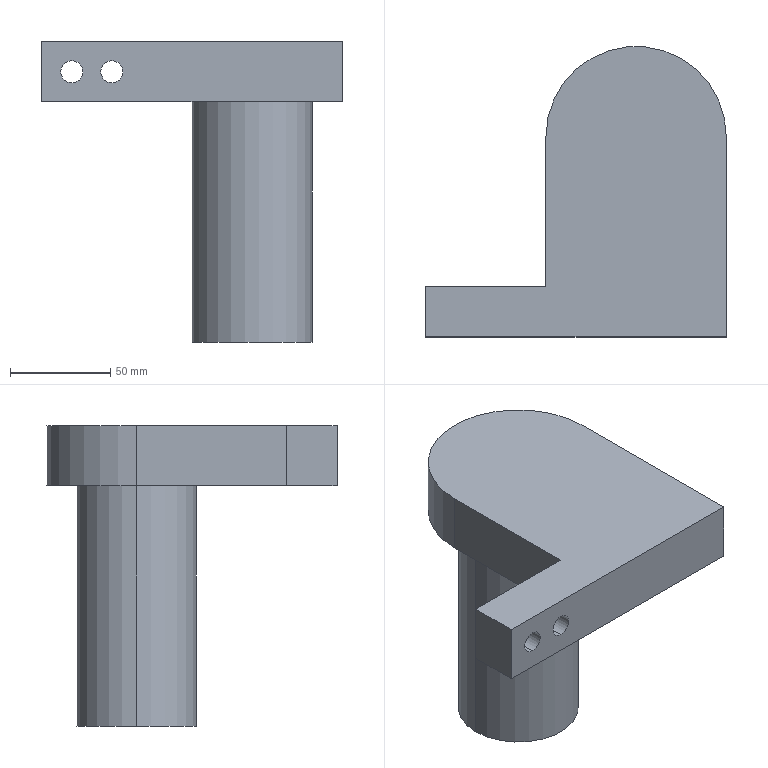Part | SolidWorks | features ICE 3, Extrusion 1 | 1 solid | 15 faces | box 150 x 145 x 150 mm | volume 744966 mm3 | plane 8 | cylinder 7 | commonest cylinder face diameters 11 x4 60 x2 90 x1
STEP:
#1=CARTESIAN_POINT('',(0.,87.5,-135.));
#2=VERTEX_POINT('',#1);
#3=CARTESIAN_POINT('',(60.,87.5,-135.));
#4=VERTEX_POINT('',#3);
#5=CARTESIAN_POINT('',(30.,87.5,-135.));
#6=DIRECTION('',(0.,0.,-1.));
#7=DIRECTION('',(-1.,0.,0.));
#8=AXIS2_PLACEMENT_3D('',#5,#6,#7);
#9=CIRCLE('',#8,30.);
#10=EDGE_CURVE('',#2,#4,#9,.T.);
#11=ORIENTED_EDGE('',*,*,#10,.F.);
#12=CARTESIAN_POINT('',(0.,87.5,-15.));
#13=VERTEX_POINT('',#12);
#14=CARTESIAN_POINT('',(0.,87.5,-135.));
#15=DIRECTION('',(0.,0.,1.));
#16=VECTOR('',#15,1000.);
#17=LINE('',#14,#16);
#18=EDGE_CURVE('',#2,#13,#17,.T.);
#19=ORIENTED_EDGE('',*,*,#18,.T.);
#20=CARTESIAN_POINT('',(60.,87.5,-15.));
#21=VERTEX_POINT('',#20);
#22=CARTESIAN_POINT('',(30.,87.5,-15.));
#23=DIRECTION('',(0.,0.,-1.));
#24=DIRECTION('',(1.,0.,0.));
#25=AXIS2_PLACEMENT_3D('',#22,#23,#24);
#26=CIRCLE('',#25,30.);
#27=EDGE_CURVE('',#13,#21,#26,.T.);
#28=ORIENTED_EDGE('',*,*,#27,.T.);
#29=CARTESIAN_POINT('',(60.,87.5,-135.));
#30=DIRECTION('',(0.,0.,1.));
#31=VECTOR('',#30,1000.);
#32=LINE('',#29,#31);
#33=EDGE_CURVE('',#4,#21,#32,.T.);
#34=ORIENTED_EDGE('',*,*,#33,.F.);
#35=EDGE_LOOP('',(#11,#19,#28,#34));
#36=FACE_OUTER_BOUND('',#35,.T.);
#37=CARTESIAN_POINT('',(30.,87.5,-135.));
#38=DIRECTION('',(0.,0.,1.));
#39=DIRECTION('',(1.,0.,0.));
#40=AXIS2_PLACEMENT_3D('',#37,#38,#39);
#41=CYLINDRICAL_SURFACE('',#40,30.);
#42=ADVANCED_FACE('',(#36),#41,.T.);
#43=CARTESIAN_POINT('',(-60.,-12.5,-5.5));
#44=VERTEX_POINT('',#43);
#45=CARTESIAN_POINT('',(-60.,-12.5,5.5));
#46=VERTEX_POINT('',#45);
#47=CARTESIAN_POINT('',(-60.,-12.5,0.));
#48=DIRECTION('',(0.,1.,0.));
#49=DIRECTION('',(0.,0.,1.));
#50=AXIS2_PLACEMENT_3D('',#47,#48,#49);
#51=CIRCLE('',#50,5.5);
#52=EDGE_CURVE('',#44,#46,#51,.T.);
#53=ORIENTED_EDGE('',*,*,#52,.F.);
#54=CARTESIAN_POINT('',(-60.,12.5,-5.5));
#55=VERTEX_POINT('',#54);
#56=CARTESIAN_POINT('',(-60.,-17.5,-5.5));
#57=DIRECTION('',(0.,1.,0.));
#58=VECTOR('',#57,1000.);
#59=LINE('',#56,#58);
#60=EDGE_CURVE('',#44,#55,#59,.T.);
#61=ORIENTED_EDGE('',*,*,#60,.T.);
#62=CARTESIAN_POINT('',(-60.,12.5,5.5));
#63=VERTEX_POINT('',#62);
#64=CARTESIAN_POINT('',(-60.,12.5,0.));
#65=DIRECTION('',(0.,1.,0.));
#66=DIRECTION('',(0.,0.,1.));
#67=AXIS2_PLACEMENT_3D('',#64,#65,#66);
#68=CIRCLE('',#67,5.5);
#69=EDGE_CURVE('',#55,#63,#68,.T.);
#70=ORIENTED_EDGE('',*,*,#69,.T.);
#71=CARTESIAN_POINT('',(-60.,-17.5,5.5));
#72=DIRECTION('',(0.,1.,0.));
#73=VECTOR('',#72,1000.);
#74=LINE('',#71,#73);
#75=EDGE_CURVE('',#46,#63,#74,.T.);
#76=ORIENTED_EDGE('',*,*,#75,.F.);
#77=EDGE_LOOP('',(#53,#61,#70,#76));
#78=FACE_OUTER_BOUND('',#77,.T.);
#79=CARTESIAN_POINT('',(-60.,-17.5,0.));
#80=DIRECTION('',(0.,1.,0.));
#81=DIRECTION('',(0.,0.,1.));
#82=AXIS2_PLACEMENT_3D('',#79,#80,#81);
#83=CYLINDRICAL_SURFACE('',#82,5.5);
#84=ADVANCED_FACE('',(#78),#83,.F.);
#85=CARTESIAN_POINT('',(-40.,-12.5,-5.5));
#86=VERTEX_POINT('',#85);
#87=CARTESIAN_POINT('',(-40.,-12.5,5.5));
#88=VERTEX_POINT('',#87);
#89=CARTESIAN_POINT('',(-40.,-12.5,0.));
#90=DIRECTION('',(0.,1.,0.));
#91=DIRECTION('',(0.,0.,1.));
#92=AXIS2_PLACEMENT_3D('',#89,#90,#91);
#93=CIRCLE('',#92,5.5);
#94=EDGE_CURVE('',#86,#88,#93,.T.);
#95=ORIENTED_EDGE('',*,*,#94,.F.);
#96=CARTESIAN_POINT('',(-40.,12.5,-5.5));
#97=VERTEX_POINT('',#96);
#98=CARTESIAN_POINT('',(-40.,-17.5,-5.5));
#99=DIRECTION('',(0.,1.,0.));
#100=VECTOR('',#99,1000.);
#101=LINE('',#98,#100);
#102=EDGE_CURVE('',#86,#97,#101,.T.);
#103=ORIENTED_EDGE('',*,*,#102,.T.);
#104=CARTESIAN_POINT('',(-40.,12.5,5.5));
#105=VERTEX_POINT('',#104);
#106=CARTESIAN_POINT('',(-40.,12.5,0.));
#107=DIRECTION('',(0.,1.,0.));
#108=DIRECTION('',(0.,0.,1.));
#109=AXIS2_PLACEMENT_3D('',#106,#107,#108);
#110=CIRCLE('',#109,5.5);
#111=EDGE_CURVE('',#97,#105,#110,.T.);
#112=ORIENTED_EDGE('',*,*,#111,.T.);
#113=CARTESIAN_POINT('',(-40.,-17.5,5.5));
#114=DIRECTION('',(0.,1.,0.));
#115=VECTOR('',#114,1000.);
#116=LINE('',#113,#115);
#117=EDGE_CURVE('',#88,#105,#116,.T.);
#118=ORIENTED_EDGE('',*,*,#117,.F.);
#119=EDGE_LOOP('',(#95,#103,#112,#118));
#120=FACE_OUTER_BOUND('',#119,.T.);
#121=CARTESIAN_POINT('',(-40.,-17.5,0.));
#122=DIRECTION('',(0.,1.,0.));
#123=DIRECTION('',(0.,0.,1.));
#124=AXIS2_PLACEMENT_3D('',#121,#122,#123);
#125=CYLINDRICAL_SURFACE('',#124,5.5);
#126=ADVANCED_FACE('',(#120),#125,.F.);
#127=CARTESIAN_POINT('',(75.,-12.5,-15.));
#128=VERTEX_POINT('',#127);
#129=CARTESIAN_POINT('',(75.,87.5,-15.));
#130=VERTEX_POINT('',#129);
#131=CARTESIAN_POINT('',(75.,12.5,-15.));
#132=DIRECTION('',(0.,1.,0.));
#133=VECTOR('',#132,1000.);
#134=LINE('',#131,#133);
#135=EDGE_CURVE('',#128,#130,#134,.T.);
#136=ORIENTED_EDGE('',*,*,#135,.T.);
#137=CARTESIAN_POINT('',(75.,87.5,15.));
#138=VERTEX_POINT('',#137);
#139=CARTESIAN_POINT('',(75.,87.5,-175.176));
#140=DIRECTION('',(0.,0.,1.));
#141=VECTOR('',#140,1000.);
#142=LINE('',#139,#141);
#143=EDGE_CURVE('',#130,#138,#142,.T.);
#144=ORIENTED_EDGE('',*,*,#143,.T.);
#145=CARTESIAN_POINT('',(75.,-12.5,15.));
#146=VERTEX_POINT('',#145);
#147=CARTESIAN_POINT('',(75.,12.5,15.));
#148=DIRECTION('',(0.,1.,0.));
#149=VECTOR('',#148,1000.);
#150=LINE('',#147,#149);
#151=EDGE_CURVE('',#146,#138,#150,.T.);
#152=ORIENTED_EDGE('',*,*,#151,.F.);
#153=CARTESIAN_POINT('',(75.,-12.5,15.));
#154=DIRECTION('',(0.,0.,-1.));
#155=VECTOR('',#154,1000.);
#156=LINE('',#153,#155);
#157=EDGE_CURVE('',#146,#128,#156,.T.);
#158=ORIENTED_EDGE('',*,*,#157,.T.);
#159=EDGE_LOOP('',(#136,#144,#152,#158));
#160=FACE_OUTER_BOUND('',#159,.T.);
#161=CARTESIAN_POINT('',(75.,12.5,15.));
#162=DIRECTION('',(-1.,0.,0.));
#163=DIRECTION('',(0.,0.,1.));
#164=AXIS2_PLACEMENT_3D('',#161,#162,#163);
#165=PLANE('',#164);
#166=ADVANCED_FACE('',(#160),#165,.F.);
#167=CARTESIAN_POINT('',(-60.,12.5,0.));
#168=DIRECTION('',(0.,1.,0.));
#169=DIRECTION('',(0.,0.,1.));
#170=AXIS2_PLACEMENT_3D('',#167,#168,#169);
#171=CIRCLE('',#170,5.5);
#172=EDGE_CURVE('',#63,#55,#171,.T.);
#173=ORIENTED_EDGE('',*,*,#172,.F.);
#174=ORIENTED_EDGE('',*,*,#69,.F.);
#175=EDGE_LOOP('',(#173,#174));
#176=FACE_BOUND('',#175,.T.);
#177=CARTESIAN_POINT('',(-40.,12.5,0.));
#178=DIRECTION('',(0.,1.,0.));
#179=DIRECTION('',(0.,0.,1.));
#180=AXIS2_PLACEMENT_3D('',#177,#178,#179);
#181=CIRCLE('',#180,5.5);
#182=EDGE_CURVE('',#105,#97,#181,.T.);
#183=ORIENTED_EDGE('',*,*,#182,.F.);
#184=ORIENTED_EDGE('',*,*,#111,.F.);
#185=EDGE_LOOP('',(#183,#184));
#186=FACE_BOUND('',#185,.T.);
#187=CARTESIAN_POINT('',(-15.,12.5,15.));
#188=VERTEX_POINT('',#187);
#189=CARTESIAN_POINT('',(-75.,12.5,15.));
#190=VERTEX_POINT('',#189);
#191=CARTESIAN_POINT('',(-75.,12.5,15.));
#192=DIRECTION('',(-1.,0.,0.));
#193=VECTOR('',#192,1000.);
#194=LINE('',#191,#193);
#195=EDGE_CURVE('',#188,#190,#194,.T.);
#196=ORIENTED_EDGE('',*,*,#195,.F.);
#197=CARTESIAN_POINT('',(-15.,12.5,-15.));
#198=VERTEX_POINT('',#197);
#199=CARTESIAN_POINT('',(-15.,12.5,15.));
#200=DIRECTION('',(0.,0.,-1.));
#201=VECTOR('',#200,1000.);
#202=LINE('',#199,#201);
#203=EDGE_CURVE('',#188,#198,#202,.T.);
#204=ORIENTED_EDGE('',*,*,#203,.T.);
#205=CARTESIAN_POINT('',(-75.,12.5,-15.));
#206=VERTEX_POINT('',#205);
#207=CARTESIAN_POINT('',(-75.,12.5,-15.));
#208=DIRECTION('',(-1.,0.,0.));
#209=VECTOR('',#208,1000.);
#210=LINE('',#207,#209);
#211=EDGE_CURVE('',#198,#206,#210,.T.);
#212=ORIENTED_EDGE('',*,*,#211,.T.);
#213=CARTESIAN_POINT('',(-75.,12.5,15.));
#214=DIRECTION('',(0.,0.,-1.));
#215=VECTOR('',#214,1000.);
#216=LINE('',#213,#215);
#217=EDGE_CURVE('',#190,#206,#216,.T.);
#218=ORIENTED_EDGE('',*,*,#217,.F.);
#219=EDGE_LOOP('',(#196,#204,#212,#218));
#220=FACE_OUTER_BOUND('',#219,.T.);
#221=CARTESIAN_POINT('',(-75.,12.5,15.));
#222=DIRECTION('',(0.,-1.,0.));
#223=DIRECTION('',(0.,0.,-1.));
#224=AXIS2_PLACEMENT_3D('',#221,#222,#223);
#225=PLANE('',#224);
#226=ADVANCED_FACE('',(#176,#186,#220),#225,.F.);
#227=CARTESIAN_POINT('',(-75.,-12.5,-15.));
#228=VERTEX_POINT('',#227);
#229=CARTESIAN_POINT('',(-75.,12.5,-15.));
#230=DIRECTION('',(0.,-1.,0.));
#231=VECTOR('',#230,1000.);
#232=LINE('',#229,#231);
#233=EDGE_CURVE('',#206,#228,#232,.T.);
#234=ORIENTED_EDGE('',*,*,#233,.T.);
#235=CARTESIAN_POINT('',(-75.,-12.5,15.));
#236=VERTEX_POINT('',#235);
#237=CARTESIAN_POINT('',(-75.,-12.5,15.));
#238=DIRECTION('',(0.,0.,-1.));
#239=VECTOR('',#238,1000.);
#240=LINE('',#237,#239);
#241=EDGE_CURVE('',#236,#228,#240,.T.);
#242=ORIENTED_EDGE('',*,*,#241,.F.);
#243=CARTESIAN_POINT('',(-75.,12.5,15.));
#244=DIRECTION('',(0.,-1.,0.));
#245=VECTOR('',#244,1000.);
#246=LINE('',#243,#245);
#247=EDGE_CURVE('',#190,#236,#246,.T.);
#248=ORIENTED_EDGE('',*,*,#247,.F.);
#249=ORIENTED_EDGE('',*,*,#217,.T.);
#250=EDGE_LOOP('',(#234,#242,#248,#249));
#251=FACE_OUTER_BOUND('',#250,.T.);
#252=CARTESIAN_POINT('',(-75.,12.5,15.));
#253=DIRECTION('',(1.,0.,0.));
#254=DIRECTION('',(0.,0.,-1.));
#255=AXIS2_PLACEMENT_3D('',#252,#253,#254);
#256=PLANE('',#255);
#257=ADVANCED_FACE('',(#251),#256,.F.);
#258=CARTESIAN_POINT('',(-60.,-12.5,0.));
#259=DIRECTION('',(0.,1.,0.));
#260=DIRECTION('',(0.,0.,1.));
#261=AXIS2_PLACEMENT_3D('',#258,#259,#260);
#262=CIRCLE('',#261,5.5);
#263=EDGE_CURVE('',#46,#44,#262,.T.);
#264=ORIENTED_EDGE('',*,*,#263,.T.);
#265=ORIENTED_EDGE('',*,*,#52,.T.);
#266=EDGE_LOOP('',(#264,#265));
#267=FACE_BOUND('',#266,.T.);
#268=CARTESIAN_POINT('',(-40.,-12.5,0.));
#269=DIRECTION('',(0.,1.,0.));
#270=DIRECTION('',(0.,0.,1.));
#271=AXIS2_PLACEMENT_3D('',#268,#269,#270);
#272=CIRCLE('',#271,5.5);
#273=EDGE_CURVE('',#88,#86,#272,.T.);
#274=ORIENTED_EDGE('',*,*,#273,.T.);
#275=ORIENTED_EDGE('',*,*,#94,.T.);
#276=EDGE_LOOP('',(#274,#275));
#277=FACE_BOUND('',#276,.T.);
#278=CARTESIAN_POINT('',(-75.,-12.5,-15.));
#279=DIRECTION('',(1.,0.,0.));
#280=VECTOR('',#279,1000.);
#281=LINE('',#278,#280);
#282=EDGE_CURVE('',#228,#128,#281,.T.);
#283=ORIENTED_EDGE('',*,*,#282,.T.);
#284=ORIENTED_EDGE('',*,*,#157,.F.);
#285=CARTESIAN_POINT('',(-75.,-12.5,15.));
#286=DIRECTION('',(1.,0.,0.));
#287=VECTOR('',#286,1000.);
#288=LINE('',#285,#287);
#289=EDGE_CURVE('',#236,#146,#288,.T.);
#290=ORIENTED_EDGE('',*,*,#289,.F.);
#291=ORIENTED_EDGE('',*,*,#241,.T.);
#292=EDGE_LOOP('',(#283,#284,#290,#291));
#293=FACE_OUTER_BOUND('',#292,.T.);
#294=CARTESIAN_POINT('',(-75.,-12.5,15.));
#295=DIRECTION('',(0.,1.,0.));
#296=DIRECTION('',(0.,0.,1.));
#297=AXIS2_PLACEMENT_3D('',#294,#295,#296);
#298=PLANE('',#297);
#299=ADVANCED_FACE('',(#267,#277,#293),#298,.F.);
#300=ORIENTED_EDGE('',*,*,#151,.T.);
#301=CARTESIAN_POINT('',(-15.,87.5,15.));
#302=VERTEX_POINT('',#301);
#303=CARTESIAN_POINT('',(30.,87.5,15.));
#304=DIRECTION('',(0.,0.,1.));
#305=DIRECTION('',(1.,0.,0.));
#306=AXIS2_PLACEMENT_3D('',#303,#304,#305);
#307=CIRCLE('',#306,45.);
#308=EDGE_CURVE('',#138,#302,#307,.T.);
#309=ORIENTED_EDGE('',*,*,#308,.T.);
#310=CARTESIAN_POINT('',(-15.,87.5,15.));
#311=DIRECTION('',(0.,-1.,0.));
#312=VECTOR('',#311,1000.);
#313=LINE('',#310,#312);
#314=EDGE_CURVE('',#302,#188,#313,.T.);
#315=ORIENTED_EDGE('',*,*,#314,.T.);
#316=ORIENTED_EDGE('',*,*,#195,.T.);
#317=ORIENTED_EDGE('',*,*,#247,.T.);
#318=ORIENTED_EDGE('',*,*,#289,.T.);
#319=EDGE_LOOP('',(#300,#309,#315,#316,#317,#318));
#320=FACE_OUTER_BOUND('',#319,.T.);
#321=CARTESIAN_POINT('',(0.,0.,15.));
#322=DIRECTION('',(0.,0.,1.));
#323=DIRECTION('',(1.,0.,0.));
#324=AXIS2_PLACEMENT_3D('',#321,#322,#323);
#325=PLANE('',#324);
#326=ADVANCED_FACE('',(#320),#325,.T.);
#327=ORIENTED_EDGE('',*,*,#211,.F.);
#328=CARTESIAN_POINT('',(-15.,87.5,-15.));
#329=VERTEX_POINT('',#328);
#330=CARTESIAN_POINT('',(-15.,87.5,-15.));
#331=DIRECTION('',(0.,1.,0.));
#332=VECTOR('',#331,1000.);
#333=LINE('',#330,#332);
#334=EDGE_CURVE('',#198,#329,#333,.T.);
#335=ORIENTED_EDGE('',*,*,#334,.T.);
#336=CARTESIAN_POINT('',(30.,87.5,-15.));
#337=DIRECTION('',(0.,0.,-1.));
#338=DIRECTION('',(1.,0.,0.));
#339=AXIS2_PLACEMENT_3D('',#336,#337,#338);
#340=CIRCLE('',#339,45.);
#341=EDGE_CURVE('',#329,#130,#340,.T.);
#342=ORIENTED_EDGE('',*,*,#341,.T.);
#343=ORIENTED_EDGE('',*,*,#135,.F.);
#344=ORIENTED_EDGE('',*,*,#282,.F.);
#345=ORIENTED_EDGE('',*,*,#233,.F.);
#346=EDGE_LOOP('',(#327,#335,#342,#343,#344,#345));
#347=FACE_OUTER_BOUND('',#346,.T.);
#348=CARTESIAN_POINT('',(30.,87.5,-15.));
#349=DIRECTION('',(0.,0.,-1.));
#350=DIRECTION('',(1.,0.,0.));
#351=AXIS2_PLACEMENT_3D('',#348,#349,#350);
#352=CIRCLE('',#351,30.);
#353=EDGE_CURVE('',#21,#13,#352,.T.);
#354=ORIENTED_EDGE('',*,*,#353,.F.);
#355=ORIENTED_EDGE('',*,*,#27,.F.);
#356=EDGE_LOOP('',(#354,#355));
#357=FACE_BOUND('',#356,.T.);
#358=CARTESIAN_POINT('',(0.,0.,-15.));
#359=DIRECTION('',(0.,0.,1.));
#360=DIRECTION('',(1.,0.,0.));
#361=AXIS2_PLACEMENT_3D('',#358,#359,#360);
#362=PLANE('',#361);
#363=ADVANCED_FACE('',(#347,#357),#362,.F.);
#364=ORIENTED_EDGE('',*,*,#203,.F.);
#365=ORIENTED_EDGE('',*,*,#314,.F.);
#366=CARTESIAN_POINT('',(-15.,87.5,-175.176));
#367=DIRECTION('',(0.,0.,1.));
#368=VECTOR('',#367,1000.);
#369=LINE('',#366,#368);
#370=EDGE_CURVE('',#329,#302,#369,.T.);
#371=ORIENTED_EDGE('',*,*,#370,.F.);
#372=ORIENTED_EDGE('',*,*,#334,.F.);
#373=EDGE_LOOP('',(#364,#365,#371,#372));
#374=FACE_OUTER_BOUND('',#373,.T.);
#375=CARTESIAN_POINT('',(-15.,87.5,-175.176));
#376=DIRECTION('',(-1.,0.,0.));
#377=DIRECTION('',(0.,0.,1.));
#378=AXIS2_PLACEMENT_3D('',#375,#376,#377);
#379=PLANE('',#378);
#380=ADVANCED_FACE('',(#374),#379,.T.);
#381=ORIENTED_EDGE('',*,*,#341,.F.);
#382=ORIENTED_EDGE('',*,*,#370,.T.);
#383=ORIENTED_EDGE('',*,*,#308,.F.);
#384=ORIENTED_EDGE('',*,*,#143,.F.);
#385=EDGE_LOOP('',(#381,#382,#383,#384));
#386=FACE_OUTER_BOUND('',#385,.T.);
#387=CARTESIAN_POINT('',(30.,87.5,-175.176));
#388=DIRECTION('',(0.,0.,1.));
#389=DIRECTION('',(1.,0.,0.));
#390=AXIS2_PLACEMENT_3D('',#387,#388,#389);
#391=CYLINDRICAL_SURFACE('',#390,45.);
#392=ADVANCED_FACE('',(#386),#391,.T.);
#393=ORIENTED_EDGE('',*,*,#102,.F.);
#394=ORIENTED_EDGE('',*,*,#273,.F.);
#395=ORIENTED_EDGE('',*,*,#117,.T.);
#396=ORIENTED_EDGE('',*,*,#182,.T.);
#397=EDGE_LOOP('',(#393,#394,#395,#396));
#398=FACE_OUTER_BOUND('',#397,.T.);
#399=CARTESIAN_POINT('',(-40.,-17.5,0.));
#400=DIRECTION('',(0.,1.,0.));
#401=DIRECTION('',(0.,0.,1.));
#402=AXIS2_PLACEMENT_3D('',#399,#400,#401);
#403=CYLINDRICAL_SURFACE('',#402,5.5);
#404=ADVANCED_FACE('',(#398),#403,.F.);
#405=ORIENTED_EDGE('',*,*,#60,.F.);
#406=ORIENTED_EDGE('',*,*,#263,.F.);
#407=ORIENTED_EDGE('',*,*,#75,.T.);
#408=ORIENTED_EDGE('',*,*,#172,.T.);
#409=EDGE_LOOP('',(#405,#406,#407,#408));
#410=FACE_OUTER_BOUND('',#409,.T.);
#411=CARTESIAN_POINT('',(-60.,-17.5,0.));
#412=DIRECTION('',(0.,1.,0.));
#413=DIRECTION('',(0.,0.,1.));
#414=AXIS2_PLACEMENT_3D('',#411,#412,#413);
#415=CYLINDRICAL_SURFACE('',#414,5.5);
#416=ADVANCED_FACE('',(#410),#415,.F.);
#417=ORIENTED_EDGE('',*,*,#18,.F.);
#418=CARTESIAN_POINT('',(30.,87.5,-135.));
#419=DIRECTION('',(0.,0.,-1.));
#420=DIRECTION('',(-1.,0.,0.));
#421=AXIS2_PLACEMENT_3D('',#418,#419,#420);
#422=CIRCLE('',#421,30.);
#423=EDGE_CURVE('',#4,#2,#422,.T.);
#424=ORIENTED_EDGE('',*,*,#423,.F.);
#425=ORIENTED_EDGE('',*,*,#33,.T.);
#426=ORIENTED_EDGE('',*,*,#353,.T.);
#427=EDGE_LOOP('',(#417,#424,#425,#426));
#428=FACE_OUTER_BOUND('',#427,.T.);
#429=CARTESIAN_POINT('',(30.,87.5,-135.));
#430=DIRECTION('',(0.,0.,1.));
#431=DIRECTION('',(1.,0.,0.));
#432=AXIS2_PLACEMENT_3D('',#429,#430,#431);
#433=CYLINDRICAL_SURFACE('',#432,30.);
#434=ADVANCED_FACE('',(#428),#433,.T.);
#435=ORIENTED_EDGE('',*,*,#423,.T.);
#436=ORIENTED_EDGE('',*,*,#10,.T.);
#437=EDGE_LOOP('',(#435,#436));
#438=FACE_OUTER_BOUND('',#437,.T.);
#439=CARTESIAN_POINT('',(30.,87.5,-135.));
#440=DIRECTION('',(0.,0.,-1.));
#441=DIRECTION('',(-1.,0.,0.));
#442=AXIS2_PLACEMENT_3D('',#439,#440,#441);
#443=PLANE('',#442);
#444=ADVANCED_FACE('',(#438),#443,.T.);
#445=CLOSED_SHELL('',(#42,#84,#126,#166,#226,#257,#299,#326,#363,#380,#392,#404,#416,#434,#444));
#446=MANIFOLD_SOLID_BREP('',#445);
#447=CARTESIAN_POINT('',(0.,0.,0.));
#448=DIRECTION('',(0.,0.,1.));
#449=DIRECTION('',(1.,0.,0.));
#450=AXIS2_PLACEMENT_3D('',#447,#448,#449);
#451=(LENGTH_UNIT()NAMED_UNIT(*)SI_UNIT(.MILLI.,.METRE.));
#452=UNCERTAINTY_MEASURE_WITH_UNIT(LENGTH_MEASURE(0.00001),#451,'','');
#453=(NAMED_UNIT(*)PLANE_ANGLE_UNIT()SI_UNIT($,.RADIAN.));
#454=(NAMED_UNIT(*)SI_UNIT($,.STERADIAN.)SOLID_ANGLE_UNIT());
#455=(GEOMETRIC_REPRESENTATION_CONTEXT(3)GLOBAL_UNCERTAINTY_ASSIGNED_CONTEXT((#452))GLOBAL_UNIT_ASSIGNED_CONTEXT((#451,#453,#454))REPRESENTATION_CONTEXT('',''));
#456=ADVANCED_BREP_SHAPE_REPRESENTATION('',(#446,#450),#455);